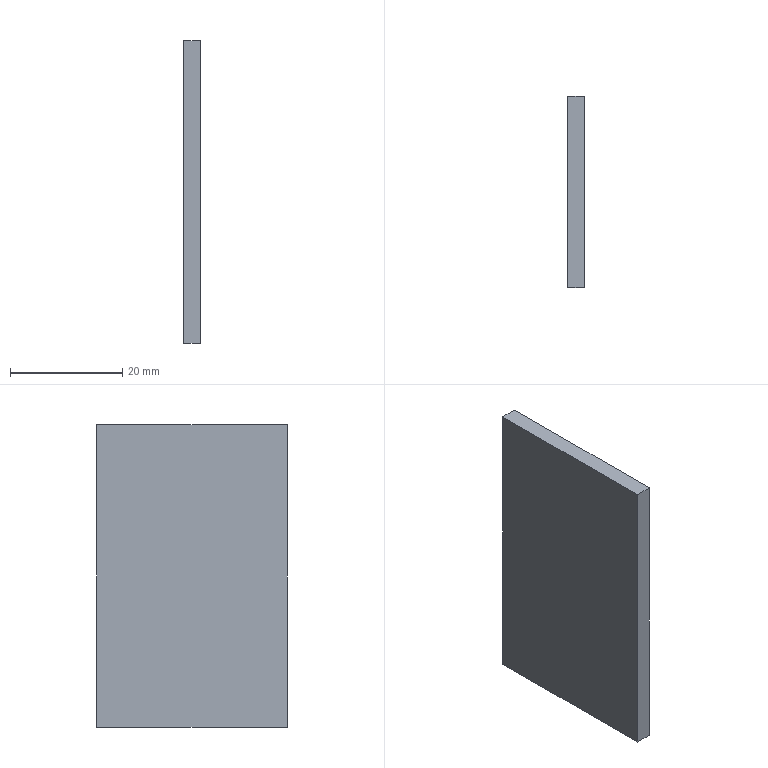Part | STEP file | HL4GD-1.30.114_60×40封Plate--20251212 | 1 solid | 6 faces | box 3 x 34 x 54 mm | volume 5508 mm3 | plane 6
STEP:
#1=CARTESIAN_POINT('',(0.,0.,0.));
#2=DIRECTION('',(0.,0.,1.));
#3=DIRECTION('',(1.,0.,0.));
#4=AXIS2_PLACEMENT_3D('',#1,#2,#3);
#5=CARTESIAN_POINT('',(1515.,1113.,408.));
#6=VERTEX_POINT('',#5);
#7=CARTESIAN_POINT('',(1515.,1113.,462.));
#8=VERTEX_POINT('',#7);
#9=CARTESIAN_POINT('',(1515.,1113.,415.));
#10=DIRECTION('',(0.,0.,1.));
#11=VECTOR('',#10,1.);
#12=LINE('',#9,#11);
#13=CARTESIAN_POINT('',(1512.,1113.,415.));
#14=DIRECTION('',(0.,1.,0.));
#15=DIRECTION('',(0.,0.,1.));
#16=AXIS2_PLACEMENT_3D('',#13,#14,#15);
#17=PLANE('',#16);
#18=CARTESIAN_POINT('',(0.,3.));
#19=DIRECTION('',(1.,0.));
#20=VECTOR('',#19,1.);
#21=LINE('',#18,#20);
#22=(GEOMETRIC_REPRESENTATION_CONTEXT(2)PARAMETRIC_REPRESENTATION_CONTEXT()REPRESENTATION_CONTEXT('',''));
#23=DEFINITIONAL_REPRESENTATION('',(#21),#22);
#24=PCURVE('',#17,#23);
#25=CARTESIAN_POINT('',(1515.,1120.,455.));
#26=DIRECTION('',(-1.,0.,0.));
#27=DIRECTION('',(0.,0.,1.));
#28=AXIS2_PLACEMENT_3D('',#25,#26,#27);
#29=PLANE('',#28);
#30=CARTESIAN_POINT('',(-40.,-7.));
#31=DIRECTION('',(1.,0.));
#32=VECTOR('',#31,1.);
#33=LINE('',#30,#32);
#34=(GEOMETRIC_REPRESENTATION_CONTEXT(2)PARAMETRIC_REPRESENTATION_CONTEXT()REPRESENTATION_CONTEXT('',''));
#35=DEFINITIONAL_REPRESENTATION('',(#33),#34);
#36=PCURVE('',#29,#35);
#37=SURFACE_CURVE('',#12,(#24,#36),.PCURVE_S1.);
#38=EDGE_CURVE('',#6,#8,#37,.T.);
#39=ORIENTED_EDGE('',*,*,#38,.T.);
#40=CARTESIAN_POINT('',(1512.,1113.,462.));
#41=VERTEX_POINT('',#40);
#42=CARTESIAN_POINT('',(1512.,1113.,462.));
#43=DIRECTION('',(1.,0.,0.));
#44=VECTOR('',#43,1.);
#45=LINE('',#42,#44);
#46=CARTESIAN_POINT('',(47.,0.));
#47=DIRECTION('',(0.,1.));
#48=VECTOR('',#47,1.);
#49=LINE('',#46,#48);
#50=(GEOMETRIC_REPRESENTATION_CONTEXT(2)PARAMETRIC_REPRESENTATION_CONTEXT()REPRESENTATION_CONTEXT('',''));
#51=DEFINITIONAL_REPRESENTATION('',(#49),#50);
#52=PCURVE('',#17,#51);
#53=CARTESIAN_POINT('',(1512.,1120.,462.));
#54=DIRECTION('',(0.,0.,-1.));
#55=DIRECTION('',(0.,1.,0.));
#56=AXIS2_PLACEMENT_3D('',#53,#54,#55);
#57=PLANE('',#56);
#58=CARTESIAN_POINT('',(-7.,0.));
#59=DIRECTION('',(0.,1.));
#60=VECTOR('',#59,1.);
#61=LINE('',#58,#60);
#62=(GEOMETRIC_REPRESENTATION_CONTEXT(2)PARAMETRIC_REPRESENTATION_CONTEXT()REPRESENTATION_CONTEXT('',''));
#63=DEFINITIONAL_REPRESENTATION('',(#61),#62);
#64=PCURVE('',#57,#63);
#65=SURFACE_CURVE('',#45,(#52,#64),.PCURVE_S1.);
#66=EDGE_CURVE('',#41,#8,#65,.T.);
#67=ORIENTED_EDGE('',*,*,#66,.F.);
#68=CARTESIAN_POINT('',(1512.,1113.,408.));
#69=VERTEX_POINT('',#68);
#70=CARTESIAN_POINT('',(1512.,1113.,415.));
#71=DIRECTION('',(0.,0.,1.));
#72=VECTOR('',#71,1.);
#73=LINE('',#70,#72);
#74=CARTESIAN_POINT('',(0.,0.));
#75=DIRECTION('',(1.,0.));
#76=VECTOR('',#75,1.);
#77=LINE('',#74,#76);
#78=(GEOMETRIC_REPRESENTATION_CONTEXT(2)PARAMETRIC_REPRESENTATION_CONTEXT()REPRESENTATION_CONTEXT('',''));
#79=DEFINITIONAL_REPRESENTATION('',(#77),#78);
#80=PCURVE('',#17,#79);
#81=CARTESIAN_POINT('',(1512.,1120.,455.));
#82=DIRECTION('',(-1.,0.,0.));
#83=DIRECTION('',(0.,0.,1.));
#84=AXIS2_PLACEMENT_3D('',#81,#82,#83);
#85=PLANE('',#84);
#86=CARTESIAN_POINT('',(-40.,-7.));
#87=DIRECTION('',(1.,0.));
#88=VECTOR('',#87,1.);
#89=LINE('',#86,#88);
#90=(GEOMETRIC_REPRESENTATION_CONTEXT(2)PARAMETRIC_REPRESENTATION_CONTEXT()REPRESENTATION_CONTEXT('',''));
#91=DEFINITIONAL_REPRESENTATION('',(#89),#90);
#92=PCURVE('',#85,#91);
#93=SURFACE_CURVE('',#73,(#80,#92),.PCURVE_S1.);
#94=EDGE_CURVE('',#69,#41,#93,.T.);
#95=ORIENTED_EDGE('',*,*,#94,.F.);
#96=CARTESIAN_POINT('',(1512.,1113.,408.));
#97=DIRECTION('',(1.,0.,0.));
#98=VECTOR('',#97,1.);
#99=LINE('',#96,#98);
#100=CARTESIAN_POINT('',(-7.,0.));
#101=DIRECTION('',(0.,1.));
#102=VECTOR('',#101,1.);
#103=LINE('',#100,#102);
#104=(GEOMETRIC_REPRESENTATION_CONTEXT(2)PARAMETRIC_REPRESENTATION_CONTEXT()REPRESENTATION_CONTEXT('',''));
#105=DEFINITIONAL_REPRESENTATION('',(#103),#104);
#106=PCURVE('',#17,#105);
#107=CARTESIAN_POINT('',(1512.,1140.,408.));
#108=DIRECTION('',(0.,0.,1.));
#109=DIRECTION('',(0.,-1.,0.));
#110=AXIS2_PLACEMENT_3D('',#107,#108,#109);
#111=PLANE('',#110);
#112=CARTESIAN_POINT('',(27.,0.));
#113=DIRECTION('',(0.,1.));
#114=VECTOR('',#113,1.);
#115=LINE('',#112,#114);
#116=(GEOMETRIC_REPRESENTATION_CONTEXT(2)PARAMETRIC_REPRESENTATION_CONTEXT()REPRESENTATION_CONTEXT('',''));
#117=DEFINITIONAL_REPRESENTATION('',(#115),#116);
#118=PCURVE('',#111,#117);
#119=SURFACE_CURVE('',#99,(#106,#118),.PCURVE_S1.);
#120=EDGE_CURVE('',#69,#6,#119,.T.);
#121=ORIENTED_EDGE('',*,*,#120,.T.);
#122=EDGE_LOOP('',(#39,#67,#95,#121));
#123=FACE_BOUND('',#122,.T.);
#124=ADVANCED_FACE('',(#123),#17,.F.);
#125=CARTESIAN_POINT('',(1515.,1147.,462.));
#126=VERTEX_POINT('',#125);
#127=CARTESIAN_POINT('',(1515.,1120.,462.));
#128=DIRECTION('',(0.,1.,0.));
#129=VECTOR('',#128,1.);
#130=LINE('',#127,#129);
#131=CARTESIAN_POINT('',(0.,3.));
#132=DIRECTION('',(1.,0.));
#133=VECTOR('',#132,1.);
#134=LINE('',#131,#133);
#135=(GEOMETRIC_REPRESENTATION_CONTEXT(2)PARAMETRIC_REPRESENTATION_CONTEXT()REPRESENTATION_CONTEXT('',''));
#136=DEFINITIONAL_REPRESENTATION('',(#134),#135);
#137=PCURVE('',#57,#136);
#138=CARTESIAN_POINT('',(7.,0.));
#139=DIRECTION('',(0.,1.));
#140=VECTOR('',#139,1.);
#141=LINE('',#138,#140);
#142=(GEOMETRIC_REPRESENTATION_CONTEXT(2)PARAMETRIC_REPRESENTATION_CONTEXT()REPRESENTATION_CONTEXT('',''));
#143=DEFINITIONAL_REPRESENTATION('',(#141),#142);
#144=PCURVE('',#29,#143);
#145=SURFACE_CURVE('',#130,(#137,#144),.PCURVE_S1.);
#146=EDGE_CURVE('',#8,#126,#145,.T.);
#147=ORIENTED_EDGE('',*,*,#146,.T.);
#148=CARTESIAN_POINT('',(1512.,1147.,462.));
#149=VERTEX_POINT('',#148);
#150=CARTESIAN_POINT('',(1512.,1147.,462.));
#151=DIRECTION('',(1.,0.,0.));
#152=VECTOR('',#151,1.);
#153=LINE('',#150,#152);
#154=CARTESIAN_POINT('',(27.,0.));
#155=DIRECTION('',(0.,1.));
#156=VECTOR('',#155,1.);
#157=LINE('',#154,#156);
#158=(GEOMETRIC_REPRESENTATION_CONTEXT(2)PARAMETRIC_REPRESENTATION_CONTEXT()REPRESENTATION_CONTEXT('',''));
#159=DEFINITIONAL_REPRESENTATION('',(#157),#158);
#160=PCURVE('',#57,#159);
#161=CARTESIAN_POINT('',(1512.,1147.,455.));
#162=DIRECTION('',(0.,-1.,0.));
#163=DIRECTION('',(0.,0.,-1.));
#164=AXIS2_PLACEMENT_3D('',#161,#162,#163);
#165=PLANE('',#164);
#166=CARTESIAN_POINT('',(-7.,0.));
#167=DIRECTION('',(0.,1.));
#168=VECTOR('',#167,1.);
#169=LINE('',#166,#168);
#170=(GEOMETRIC_REPRESENTATION_CONTEXT(2)PARAMETRIC_REPRESENTATION_CONTEXT()REPRESENTATION_CONTEXT('',''));
#171=DEFINITIONAL_REPRESENTATION('',(#169),#170);
#172=PCURVE('',#165,#171);
#173=SURFACE_CURVE('',#153,(#160,#172),.PCURVE_S1.);
#174=EDGE_CURVE('',#149,#126,#173,.T.);
#175=ORIENTED_EDGE('',*,*,#174,.F.);
#176=CARTESIAN_POINT('',(1512.,1120.,462.));
#177=DIRECTION('',(0.,1.,0.));
#178=VECTOR('',#177,1.);
#179=LINE('',#176,#178);
#180=CARTESIAN_POINT('',(0.,0.));
#181=DIRECTION('',(1.,0.));
#182=VECTOR('',#181,1.);
#183=LINE('',#180,#182);
#184=(GEOMETRIC_REPRESENTATION_CONTEXT(2)PARAMETRIC_REPRESENTATION_CONTEXT()REPRESENTATION_CONTEXT('',''));
#185=DEFINITIONAL_REPRESENTATION('',(#183),#184);
#186=PCURVE('',#57,#185);
#187=CARTESIAN_POINT('',(7.,0.));
#188=DIRECTION('',(0.,1.));
#189=VECTOR('',#188,1.);
#190=LINE('',#187,#189);
#191=(GEOMETRIC_REPRESENTATION_CONTEXT(2)PARAMETRIC_REPRESENTATION_CONTEXT()REPRESENTATION_CONTEXT('',''));
#192=DEFINITIONAL_REPRESENTATION('',(#190),#191);
#193=PCURVE('',#85,#192);
#194=SURFACE_CURVE('',#179,(#186,#193),.PCURVE_S1.);
#195=EDGE_CURVE('',#41,#149,#194,.T.);
#196=ORIENTED_EDGE('',*,*,#195,.F.);
#197=ORIENTED_EDGE('',*,*,#66,.T.);
#198=EDGE_LOOP('',(#147,#175,#196,#197));
#199=FACE_BOUND('',#198,.T.);
#200=ADVANCED_FACE('',(#199),#57,.F.);
#201=CARTESIAN_POINT('',(1515.,1147.,408.));
#202=VERTEX_POINT('',#201);
#203=CARTESIAN_POINT('',(1515.,1147.,455.));
#204=DIRECTION('',(0.,0.,-1.));
#205=VECTOR('',#204,1.);
#206=LINE('',#203,#205);
#207=CARTESIAN_POINT('',(0.,3.));
#208=DIRECTION('',(1.,0.));
#209=VECTOR('',#208,1.);
#210=LINE('',#207,#209);
#211=(GEOMETRIC_REPRESENTATION_CONTEXT(2)PARAMETRIC_REPRESENTATION_CONTEXT()REPRESENTATION_CONTEXT('',''));
#212=DEFINITIONAL_REPRESENTATION('',(#210),#211);
#213=PCURVE('',#165,#212);
#214=CARTESIAN_POINT('',(0.,27.));
#215=DIRECTION('',(-1.,0.));
#216=VECTOR('',#215,1.);
#217=LINE('',#214,#216);
#218=(GEOMETRIC_REPRESENTATION_CONTEXT(2)PARAMETRIC_REPRESENTATION_CONTEXT()REPRESENTATION_CONTEXT('',''));
#219=DEFINITIONAL_REPRESENTATION('',(#217),#218);
#220=PCURVE('',#29,#219);
#221=SURFACE_CURVE('',#206,(#213,#220),.PCURVE_S1.);
#222=EDGE_CURVE('',#126,#202,#221,.T.);
#223=ORIENTED_EDGE('',*,*,#222,.T.);
#224=CARTESIAN_POINT('',(1512.,1147.,408.));
#225=VERTEX_POINT('',#224);
#226=CARTESIAN_POINT('',(1512.,1147.,408.));
#227=DIRECTION('',(1.,0.,0.));
#228=VECTOR('',#227,1.);
#229=LINE('',#226,#228);
#230=CARTESIAN_POINT('',(47.,0.));
#231=DIRECTION('',(0.,1.));
#232=VECTOR('',#231,1.);
#233=LINE('',#230,#232);
#234=(GEOMETRIC_REPRESENTATION_CONTEXT(2)PARAMETRIC_REPRESENTATION_CONTEXT()REPRESENTATION_CONTEXT('',''));
#235=DEFINITIONAL_REPRESENTATION('',(#233),#234);
#236=PCURVE('',#165,#235);
#237=CARTESIAN_POINT('',(-7.,0.));
#238=DIRECTION('',(0.,1.));
#239=VECTOR('',#238,1.);
#240=LINE('',#237,#239);
#241=(GEOMETRIC_REPRESENTATION_CONTEXT(2)PARAMETRIC_REPRESENTATION_CONTEXT()REPRESENTATION_CONTEXT('',''));
#242=DEFINITIONAL_REPRESENTATION('',(#240),#241);
#243=PCURVE('',#111,#242);
#244=SURFACE_CURVE('',#229,(#236,#243),.PCURVE_S1.);
#245=EDGE_CURVE('',#225,#202,#244,.T.);
#246=ORIENTED_EDGE('',*,*,#245,.F.);
#247=CARTESIAN_POINT('',(1512.,1147.,455.));
#248=DIRECTION('',(0.,0.,-1.));
#249=VECTOR('',#248,1.);
#250=LINE('',#247,#249);
#251=CARTESIAN_POINT('',(0.,0.));
#252=DIRECTION('',(1.,0.));
#253=VECTOR('',#252,1.);
#254=LINE('',#251,#253);
#255=(GEOMETRIC_REPRESENTATION_CONTEXT(2)PARAMETRIC_REPRESENTATION_CONTEXT()REPRESENTATION_CONTEXT('',''));
#256=DEFINITIONAL_REPRESENTATION('',(#254),#255);
#257=PCURVE('',#165,#256);
#258=CARTESIAN_POINT('',(0.,27.));
#259=DIRECTION('',(-1.,0.));
#260=VECTOR('',#259,1.);
#261=LINE('',#258,#260);
#262=(GEOMETRIC_REPRESENTATION_CONTEXT(2)PARAMETRIC_REPRESENTATION_CONTEXT()REPRESENTATION_CONTEXT('',''));
#263=DEFINITIONAL_REPRESENTATION('',(#261),#262);
#264=PCURVE('',#85,#263);
#265=SURFACE_CURVE('',#250,(#257,#264),.PCURVE_S1.);
#266=EDGE_CURVE('',#149,#225,#265,.T.);
#267=ORIENTED_EDGE('',*,*,#266,.F.);
#268=ORIENTED_EDGE('',*,*,#174,.T.);
#269=EDGE_LOOP('',(#223,#246,#267,#268));
#270=FACE_BOUND('',#269,.T.);
#271=ADVANCED_FACE('',(#270),#165,.F.);
#272=CARTESIAN_POINT('',(1515.,1140.,408.));
#273=DIRECTION('',(0.,-1.,0.));
#274=VECTOR('',#273,1.);
#275=LINE('',#272,#274);
#276=CARTESIAN_POINT('',(0.,3.));
#277=DIRECTION('',(1.,0.));
#278=VECTOR('',#277,1.);
#279=LINE('',#276,#278);
#280=(GEOMETRIC_REPRESENTATION_CONTEXT(2)PARAMETRIC_REPRESENTATION_CONTEXT()REPRESENTATION_CONTEXT('',''));
#281=DEFINITIONAL_REPRESENTATION('',(#279),#280);
#282=PCURVE('',#111,#281);
#283=CARTESIAN_POINT('',(-47.,20.));
#284=DIRECTION('',(0.,-1.));
#285=VECTOR('',#284,1.);
#286=LINE('',#283,#285);
#287=(GEOMETRIC_REPRESENTATION_CONTEXT(2)PARAMETRIC_REPRESENTATION_CONTEXT()REPRESENTATION_CONTEXT('',''));
#288=DEFINITIONAL_REPRESENTATION('',(#286),#287);
#289=PCURVE('',#29,#288);
#290=SURFACE_CURVE('',#275,(#282,#289),.PCURVE_S1.);
#291=EDGE_CURVE('',#202,#6,#290,.T.);
#292=ORIENTED_EDGE('',*,*,#291,.T.);
#293=ORIENTED_EDGE('',*,*,#120,.F.);
#294=CARTESIAN_POINT('',(1512.,1140.,408.));
#295=DIRECTION('',(0.,-1.,0.));
#296=VECTOR('',#295,1.);
#297=LINE('',#294,#296);
#298=CARTESIAN_POINT('',(0.,0.));
#299=DIRECTION('',(1.,0.));
#300=VECTOR('',#299,1.);
#301=LINE('',#298,#300);
#302=(GEOMETRIC_REPRESENTATION_CONTEXT(2)PARAMETRIC_REPRESENTATION_CONTEXT()REPRESENTATION_CONTEXT('',''));
#303=DEFINITIONAL_REPRESENTATION('',(#301),#302);
#304=PCURVE('',#111,#303);
#305=CARTESIAN_POINT('',(-47.,20.));
#306=DIRECTION('',(0.,-1.));
#307=VECTOR('',#306,1.);
#308=LINE('',#305,#307);
#309=(GEOMETRIC_REPRESENTATION_CONTEXT(2)PARAMETRIC_REPRESENTATION_CONTEXT()REPRESENTATION_CONTEXT('',''));
#310=DEFINITIONAL_REPRESENTATION('',(#308),#309);
#311=PCURVE('',#85,#310);
#312=SURFACE_CURVE('',#297,(#304,#311),.PCURVE_S1.);
#313=EDGE_CURVE('',#225,#69,#312,.T.);
#314=ORIENTED_EDGE('',*,*,#313,.F.);
#315=ORIENTED_EDGE('',*,*,#245,.T.);
#316=EDGE_LOOP('',(#292,#293,#314,#315));
#317=FACE_BOUND('',#316,.T.);
#318=ADVANCED_FACE('',(#317),#111,.F.);
#319=ORIENTED_EDGE('',*,*,#94,.T.);
#320=ORIENTED_EDGE('',*,*,#195,.T.);
#321=ORIENTED_EDGE('',*,*,#266,.T.);
#322=ORIENTED_EDGE('',*,*,#313,.T.);
#323=EDGE_LOOP('',(#319,#320,#321,#322));
#324=FACE_BOUND('',#323,.T.);
#325=ADVANCED_FACE('',(#324),#85,.T.);
#326=ORIENTED_EDGE('',*,*,#38,.F.);
#327=ORIENTED_EDGE('',*,*,#291,.F.);
#328=ORIENTED_EDGE('',*,*,#222,.F.);
#329=ORIENTED_EDGE('',*,*,#146,.F.);
#330=EDGE_LOOP('',(#326,#327,#328,#329));
#331=FACE_BOUND('',#330,.T.);
#332=ADVANCED_FACE('',(#331),#29,.F.);
#333=CLOSED_SHELL('',(#124,#200,#271,#318,#325,#332));
#334=MANIFOLD_SOLID_BREP('',#333);
#335=(LENGTH_UNIT()NAMED_UNIT(*)SI_UNIT(.MILLI.,.METRE.));
#336=UNCERTAINTY_MEASURE_WITH_UNIT(LENGTH_MEASURE(0.0000001),#335,'','');
#337=(NAMED_UNIT(*)PLANE_ANGLE_UNIT()SI_UNIT($,.RADIAN.));
#338=(NAMED_UNIT(*)SI_UNIT($,.STERADIAN.)SOLID_ANGLE_UNIT());
#339=(GEOMETRIC_REPRESENTATION_CONTEXT(3)GLOBAL_UNCERTAINTY_ASSIGNED_CONTEXT((#336))GLOBAL_UNIT_ASSIGNED_CONTEXT((#335,#337,#338))REPRESENTATION_CONTEXT('',''));
#340=ADVANCED_BREP_SHAPE_REPRESENTATION('',(#4,#334),#339);